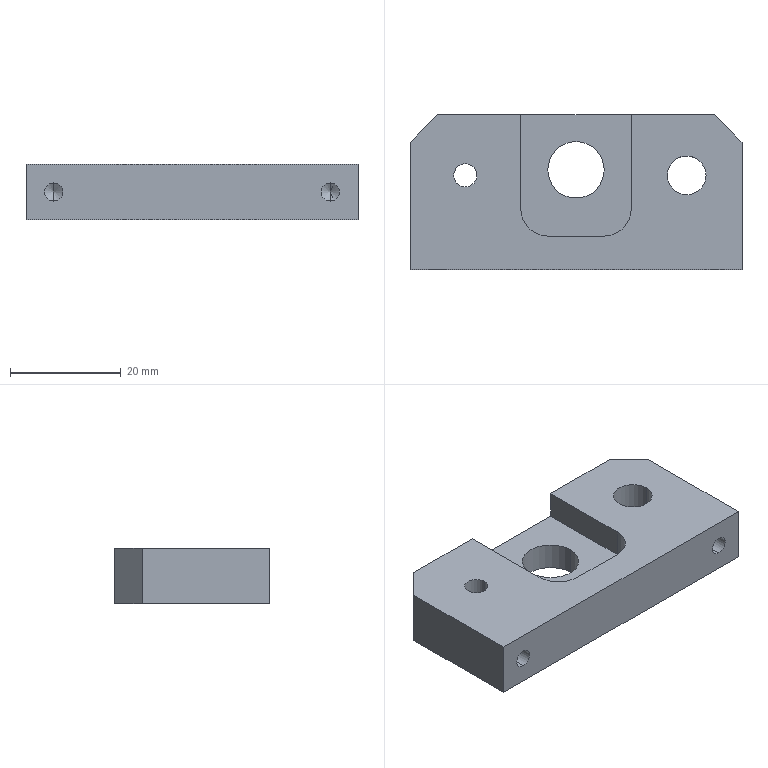Part | STEP file | PN_0048 Mount electronic clip cylinder mounting plate | 1 solid | 28 faces | box 60 x 28 x 10 mm | volume 13235 mm3 | cylinder 12 | plane 12 | cone 4 | commonest cylinder face diameters 3.3 x4 4.2 x2 7 x2 10 x2 10.2 x2